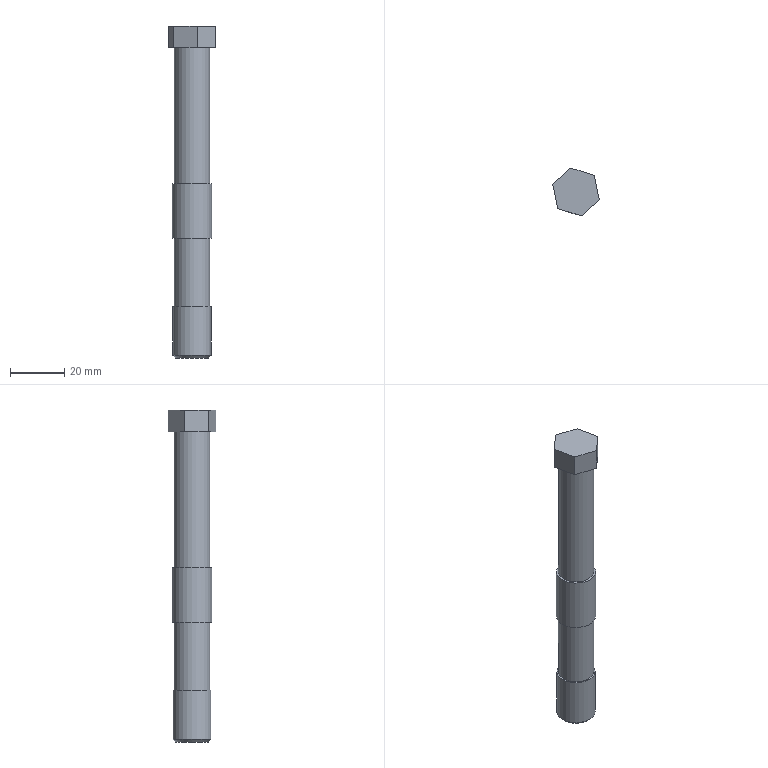Part | NX | features DATUM_CSYS 6, EXTRUDE 4, SKETCH 4, CHAMFER 1, SYMBOLIC_THREAD 1, UNITE 1 | 2 solids | 21 faces | box 17.119 x 17.607 x 122 mm | volume 18493 mm3 | plane 14 | cylinder 6 | cone 1 | commonest cylinder face diameters 13 x3 14.5 x2 14 x1
STEP:
#1=CARTESIAN_POINT('',(6.5,0.,0.));
#2=VERTEX_POINT('',#1);
#3=CARTESIAN_POINT('',(0.,0.,0.));
#4=DIRECTION('',(0.,0.,-1.));
#5=DIRECTION('',(1.,0.,0.));
#6=AXIS2_PLACEMENT_3D('',#3,#4,#5);
#7=CIRCLE('',#6,6.5);
#8=EDGE_CURVE('',#2,#2,#7,.T.);
#9=ORIENTED_EDGE('',*,*,#8,.T.);
#10=EDGE_LOOP('',(#9));
#11=FACE_BOUND('',#10,.T.);
#12=CARTESIAN_POINT('',(-6.5,0.,-50.));
#13=VERTEX_POINT('',#12);
#14=CARTESIAN_POINT('',(0.,0.,-50.));
#15=DIRECTION('',(0.,0.,-1.));
#16=DIRECTION('',(-1.,0.,0.));
#17=AXIS2_PLACEMENT_3D('',#14,#15,#16);
#18=CIRCLE('',#17,6.5);
#19=EDGE_CURVE('',#13,#13,#18,.T.);
#20=ORIENTED_EDGE('',*,*,#19,.F.);
#21=EDGE_LOOP('',(#20));
#22=FACE_BOUND('',#21,.T.);
#23=CARTESIAN_POINT('',(0.,0.,-100.));
#24=DIRECTION('',(0.,0.,1.));
#25=DIRECTION('',(1.,0.,0.));
#26=AXIS2_PLACEMENT_3D('',#23,#24,#25);
#27=CYLINDRICAL_SURFACE('',#26,6.5);
#28=ADVANCED_FACE('',(#11,#22),#27,.T.);
#29=CARTESIAN_POINT('',(1.871,-8.803,0.));
#30=VERTEX_POINT('',#29);
#31=CARTESIAN_POINT('',(8.56,-2.781,0.));
#32=VERTEX_POINT('',#31);
#33=CARTESIAN_POINT('',(1.871,-8.803,0.));
#34=DIRECTION('',(0.7431,0.6691,0.));
#35=VECTOR('',#34,1000.);
#36=LINE('',#33,#35);
#37=EDGE_CURVE('',#30,#32,#36,.T.);
#38=ORIENTED_EDGE('',*,*,#37,.F.);
#39=CARTESIAN_POINT('',(-6.688,-6.022,0.));
#40=VERTEX_POINT('',#39);
#41=CARTESIAN_POINT('',(-6.688,-6.022,0.));
#42=DIRECTION('',(0.9511,-0.309,0.));
#43=VECTOR('',#42,1000.);
#44=LINE('',#41,#43);
#45=EDGE_CURVE('',#40,#30,#44,.T.);
#46=ORIENTED_EDGE('',*,*,#45,.F.);
#47=CARTESIAN_POINT('',(-8.56,2.781,0.));
#48=VERTEX_POINT('',#47);
#49=CARTESIAN_POINT('',(-8.56,2.781,0.));
#50=DIRECTION('',(0.2079,-0.9781,0.));
#51=VECTOR('',#50,1000.);
#52=LINE('',#49,#51);
#53=EDGE_CURVE('',#48,#40,#52,.T.);
#54=ORIENTED_EDGE('',*,*,#53,.F.);
#55=CARTESIAN_POINT('',(-1.871,8.803,0.));
#56=VERTEX_POINT('',#55);
#57=CARTESIAN_POINT('',(-1.871,8.803,0.));
#58=DIRECTION('',(-0.7431,-0.6691,0.));
#59=VECTOR('',#58,1000.);
#60=LINE('',#57,#59);
#61=EDGE_CURVE('',#56,#48,#60,.T.);
#62=ORIENTED_EDGE('',*,*,#61,.F.);
#63=CARTESIAN_POINT('',(6.688,6.022,0.));
#64=VERTEX_POINT('',#63);
#65=CARTESIAN_POINT('',(6.688,6.022,0.));
#66=DIRECTION('',(-0.9511,0.309,0.));
#67=VECTOR('',#66,1000.);
#68=LINE('',#65,#67);
#69=EDGE_CURVE('',#64,#56,#68,.T.);
#70=ORIENTED_EDGE('',*,*,#69,.F.);
#71=CARTESIAN_POINT('',(8.56,-2.781,0.));
#72=DIRECTION('',(-0.2079,0.9781,0.));
#73=VECTOR('',#72,1000.);
#74=LINE('',#71,#73);
#75=EDGE_CURVE('',#32,#64,#74,.T.);
#76=ORIENTED_EDGE('',*,*,#75,.F.);
#77=EDGE_LOOP('',(#38,#46,#54,#62,#70,#76));
#78=FACE_BOUND('',#77,.T.);
#79=ORIENTED_EDGE('',*,*,#8,.F.);
#80=EDGE_LOOP('',(#79));
#81=FACE_BOUND('',#80,.T.);
#82=CARTESIAN_POINT('',(0.,0.,0.));
#83=DIRECTION('',(0.,0.,1.));
#84=DIRECTION('',(1.,0.,0.));
#85=AXIS2_PLACEMENT_3D('',#82,#83,#84);
#86=PLANE('',#85);
#87=ADVANCED_FACE('',(#78,#81),#86,.F.);
#88=ORIENTED_EDGE('',*,*,#37,.T.);
#89=CARTESIAN_POINT('',(8.56,-2.781,8.));
#90=VERTEX_POINT('',#89);
#91=CARTESIAN_POINT('',(8.56,-2.781,8.));
#92=DIRECTION('',(0.,0.,-1.));
#93=VECTOR('',#92,1000.);
#94=LINE('',#91,#93);
#95=EDGE_CURVE('',#90,#32,#94,.T.);
#96=ORIENTED_EDGE('',*,*,#95,.F.);
#97=CARTESIAN_POINT('',(1.871,-8.803,8.));
#98=VERTEX_POINT('',#97);
#99=CARTESIAN_POINT('',(1.871,-8.803,8.));
#100=DIRECTION('',(0.7431,0.6691,0.));
#101=VECTOR('',#100,1000.);
#102=LINE('',#99,#101);
#103=EDGE_CURVE('',#98,#90,#102,.T.);
#104=ORIENTED_EDGE('',*,*,#103,.F.);
#105=CARTESIAN_POINT('',(1.871,-8.803,8.));
#106=DIRECTION('',(0.,0.,-1.));
#107=VECTOR('',#106,1000.);
#108=LINE('',#105,#107);
#109=EDGE_CURVE('',#98,#30,#108,.T.);
#110=ORIENTED_EDGE('',*,*,#109,.T.);
#111=EDGE_LOOP('',(#88,#96,#104,#110));
#112=FACE_BOUND('',#111,.T.);
#113=CARTESIAN_POINT('',(1.871,-8.803,8.));
#114=DIRECTION('',(-0.6691,0.7431,0.));
#115=DIRECTION('',(-0.7431,-0.6691,0.));
#116=AXIS2_PLACEMENT_3D('',#113,#114,#115);
#117=PLANE('',#116);
#118=ADVANCED_FACE('',(#112),#117,.F.);
#119=ORIENTED_EDGE('',*,*,#75,.T.);
#120=CARTESIAN_POINT('',(6.688,6.022,8.));
#121=VERTEX_POINT('',#120);
#122=CARTESIAN_POINT('',(6.688,6.022,8.));
#123=DIRECTION('',(0.,0.,-1.));
#124=VECTOR('',#123,1000.);
#125=LINE('',#122,#124);
#126=EDGE_CURVE('',#121,#64,#125,.T.);
#127=ORIENTED_EDGE('',*,*,#126,.F.);
#128=CARTESIAN_POINT('',(8.56,-2.781,8.));
#129=DIRECTION('',(-0.2079,0.9781,0.));
#130=VECTOR('',#129,1000.);
#131=LINE('',#128,#130);
#132=EDGE_CURVE('',#90,#121,#131,.T.);
#133=ORIENTED_EDGE('',*,*,#132,.F.);
#134=ORIENTED_EDGE('',*,*,#95,.T.);
#135=EDGE_LOOP('',(#119,#127,#133,#134));
#136=FACE_BOUND('',#135,.T.);
#137=CARTESIAN_POINT('',(8.56,-2.781,8.));
#138=DIRECTION('',(-0.9781,-0.2079,0.));
#139=DIRECTION('',(0.2079,-0.9781,0.));
#140=AXIS2_PLACEMENT_3D('',#137,#138,#139);
#141=PLANE('',#140);
#142=ADVANCED_FACE('',(#136),#141,.F.);
#143=ORIENTED_EDGE('',*,*,#69,.T.);
#144=CARTESIAN_POINT('',(-1.871,8.803,8.));
#145=VERTEX_POINT('',#144);
#146=CARTESIAN_POINT('',(-1.871,8.803,8.));
#147=DIRECTION('',(0.,0.,-1.));
#148=VECTOR('',#147,1000.);
#149=LINE('',#146,#148);
#150=EDGE_CURVE('',#145,#56,#149,.T.);
#151=ORIENTED_EDGE('',*,*,#150,.F.);
#152=CARTESIAN_POINT('',(6.688,6.022,8.));
#153=DIRECTION('',(-0.9511,0.309,0.));
#154=VECTOR('',#153,1000.);
#155=LINE('',#152,#154);
#156=EDGE_CURVE('',#121,#145,#155,.T.);
#157=ORIENTED_EDGE('',*,*,#156,.F.);
#158=ORIENTED_EDGE('',*,*,#126,.T.);
#159=EDGE_LOOP('',(#143,#151,#157,#158));
#160=FACE_BOUND('',#159,.T.);
#161=CARTESIAN_POINT('',(6.688,6.022,8.));
#162=DIRECTION('',(-0.309,-0.9511,0.));
#163=DIRECTION('',(0.9511,-0.309,0.));
#164=AXIS2_PLACEMENT_3D('',#161,#162,#163);
#165=PLANE('',#164);
#166=ADVANCED_FACE('',(#160),#165,.F.);
#167=ORIENTED_EDGE('',*,*,#61,.T.);
#168=CARTESIAN_POINT('',(-8.56,2.781,8.));
#169=VERTEX_POINT('',#168);
#170=CARTESIAN_POINT('',(-8.56,2.781,8.));
#171=DIRECTION('',(0.,0.,-1.));
#172=VECTOR('',#171,1000.);
#173=LINE('',#170,#172);
#174=EDGE_CURVE('',#169,#48,#173,.T.);
#175=ORIENTED_EDGE('',*,*,#174,.F.);
#176=CARTESIAN_POINT('',(-1.871,8.803,8.));
#177=DIRECTION('',(-0.7431,-0.6691,0.));
#178=VECTOR('',#177,1000.);
#179=LINE('',#176,#178);
#180=EDGE_CURVE('',#145,#169,#179,.T.);
#181=ORIENTED_EDGE('',*,*,#180,.F.);
#182=ORIENTED_EDGE('',*,*,#150,.T.);
#183=EDGE_LOOP('',(#167,#175,#181,#182));
#184=FACE_BOUND('',#183,.T.);
#185=CARTESIAN_POINT('',(-1.871,8.803,8.));
#186=DIRECTION('',(0.6691,-0.7431,0.));
#187=DIRECTION('',(0.7431,0.6691,0.));
#188=AXIS2_PLACEMENT_3D('',#185,#186,#187);
#189=PLANE('',#188);
#190=ADVANCED_FACE('',(#184),#189,.F.);
#191=ORIENTED_EDGE('',*,*,#53,.T.);
#192=CARTESIAN_POINT('',(-6.688,-6.022,8.));
#193=VERTEX_POINT('',#192);
#194=CARTESIAN_POINT('',(-6.688,-6.022,8.));
#195=DIRECTION('',(0.,0.,-1.));
#196=VECTOR('',#195,1000.);
#197=LINE('',#194,#196);
#198=EDGE_CURVE('',#193,#40,#197,.T.);
#199=ORIENTED_EDGE('',*,*,#198,.F.);
#200=CARTESIAN_POINT('',(-8.56,2.781,8.));
#201=DIRECTION('',(0.2079,-0.9781,0.));
#202=VECTOR('',#201,1000.);
#203=LINE('',#200,#202);
#204=EDGE_CURVE('',#169,#193,#203,.T.);
#205=ORIENTED_EDGE('',*,*,#204,.F.);
#206=ORIENTED_EDGE('',*,*,#174,.T.);
#207=EDGE_LOOP('',(#191,#199,#205,#206));
#208=FACE_BOUND('',#207,.T.);
#209=CARTESIAN_POINT('',(-8.56,2.781,8.));
#210=DIRECTION('',(0.9781,0.2079,0.));
#211=DIRECTION('',(-0.2079,0.9781,0.));
#212=AXIS2_PLACEMENT_3D('',#209,#210,#211);
#213=PLANE('',#212);
#214=ADVANCED_FACE('',(#208),#213,.F.);
#215=ORIENTED_EDGE('',*,*,#45,.T.);
#216=ORIENTED_EDGE('',*,*,#109,.F.);
#217=CARTESIAN_POINT('',(-6.688,-6.022,8.));
#218=DIRECTION('',(0.9511,-0.309,0.));
#219=VECTOR('',#218,1000.);
#220=LINE('',#217,#219);
#221=EDGE_CURVE('',#193,#98,#220,.T.);
#222=ORIENTED_EDGE('',*,*,#221,.F.);
#223=ORIENTED_EDGE('',*,*,#198,.T.);
#224=EDGE_LOOP('',(#215,#216,#222,#223));
#225=FACE_BOUND('',#224,.T.);
#226=CARTESIAN_POINT('',(-6.688,-6.022,8.));
#227=DIRECTION('',(0.309,0.9511,0.));
#228=DIRECTION('',(-0.9511,0.309,0.));
#229=AXIS2_PLACEMENT_3D('',#226,#227,#228);
#230=PLANE('',#229);
#231=ADVANCED_FACE('',(#225),#230,.F.);
#232=ORIENTED_EDGE('',*,*,#103,.T.);
#233=ORIENTED_EDGE('',*,*,#132,.T.);
#234=ORIENTED_EDGE('',*,*,#156,.T.);
#235=ORIENTED_EDGE('',*,*,#180,.T.);
#236=ORIENTED_EDGE('',*,*,#204,.T.);
#237=ORIENTED_EDGE('',*,*,#221,.T.);
#238=EDGE_LOOP('',(#232,#233,#234,#235,#236,#237));
#239=FACE_BOUND('',#238,.T.);
#240=CARTESIAN_POINT('',(0.,0.,8.));
#241=DIRECTION('',(0.,0.,1.));
#242=DIRECTION('',(1.,0.,0.));
#243=AXIS2_PLACEMENT_3D('',#240,#241,#242);
#244=PLANE('',#243);
#245=ADVANCED_FACE('',(#239),#244,.T.);
#246=CARTESIAN_POINT('',(7.25,0.,-50.));
#247=VERTEX_POINT('',#246);
#248=CARTESIAN_POINT('',(0.,0.,-50.));
#249=DIRECTION('',(0.,0.,-1.));
#250=DIRECTION('',(1.,0.,0.));
#251=AXIS2_PLACEMENT_3D('',#248,#249,#250);
#252=CIRCLE('',#251,7.25);
#253=EDGE_CURVE('',#247,#247,#252,.T.);
#254=ORIENTED_EDGE('',*,*,#253,.T.);
#255=EDGE_LOOP('',(#254));
#256=FACE_BOUND('',#255,.T.);
#257=CARTESIAN_POINT('',(7.25,0.,-70.));
#258=VERTEX_POINT('',#257);
#259=CARTESIAN_POINT('',(0.,0.,-70.));
#260=DIRECTION('',(0.,0.,-1.));
#261=DIRECTION('',(1.,0.,0.));
#262=AXIS2_PLACEMENT_3D('',#259,#260,#261);
#263=CIRCLE('',#262,7.25);
#264=EDGE_CURVE('',#258,#258,#263,.T.);
#265=ORIENTED_EDGE('',*,*,#264,.F.);
#266=EDGE_LOOP('',(#265));
#267=FACE_BOUND('',#266,.T.);
#268=CARTESIAN_POINT('',(0.,0.,-50.));
#269=DIRECTION('',(0.,0.,-1.));
#270=DIRECTION('',(-1.,0.,0.));
#271=AXIS2_PLACEMENT_3D('',#268,#269,#270);
#272=CYLINDRICAL_SURFACE('',#271,7.25);
#273=ADVANCED_FACE('',(#256,#267),#272,.T.);
#274=ORIENTED_EDGE('',*,*,#253,.F.);
#275=EDGE_LOOP('',(#274));
#276=FACE_BOUND('',#275,.T.);
#277=ORIENTED_EDGE('',*,*,#19,.T.);
#278=EDGE_LOOP('',(#277));
#279=FACE_BOUND('',#278,.T.);
#280=CARTESIAN_POINT('',(0.,0.,-50.));
#281=DIRECTION('',(0.,0.,-1.));
#282=DIRECTION('',(-1.,0.,0.));
#283=AXIS2_PLACEMENT_3D('',#280,#281,#282);
#284=PLANE('',#283);
#285=ADVANCED_FACE('',(#276,#279),#284,.F.);
#286=ORIENTED_EDGE('',*,*,#264,.T.);
#287=EDGE_LOOP('',(#286));
#288=FACE_BOUND('',#287,.T.);
#289=CARTESIAN_POINT('',(6.5,0.,-70.));
#290=VERTEX_POINT('',#289);
#291=CARTESIAN_POINT('',(0.,0.,-70.));
#292=DIRECTION('',(0.,0.,-1.));
#293=DIRECTION('',(1.,0.,0.));
#294=AXIS2_PLACEMENT_3D('',#291,#292,#293);
#295=CIRCLE('',#294,6.5);
#296=EDGE_CURVE('',#290,#290,#295,.T.);
#297=ORIENTED_EDGE('',*,*,#296,.F.);
#298=EDGE_LOOP('',(#297));
#299=FACE_BOUND('',#298,.T.);
#300=CARTESIAN_POINT('',(0.,0.,-70.));
#301=DIRECTION('',(0.,0.,-1.));
#302=DIRECTION('',(-1.,0.,0.));
#303=AXIS2_PLACEMENT_3D('',#300,#301,#302);
#304=PLANE('',#303);
#305=ADVANCED_FACE('',(#288,#299),#304,.T.);
#306=CARTESIAN_POINT('',(-6.,0.,-114.));
#307=VERTEX_POINT('',#306);
#308=CARTESIAN_POINT('',(0.,0.,-114.));
#309=DIRECTION('',(0.,0.,-1.));
#310=DIRECTION('',(-1.,0.,0.));
#311=AXIS2_PLACEMENT_3D('',#308,#309,#310);
#312=CIRCLE('',#311,6.);
#313=EDGE_CURVE('',#307,#307,#312,.T.);
#314=ORIENTED_EDGE('',*,*,#313,.T.);
#315=EDGE_LOOP('',(#314));
#316=FACE_BOUND('',#315,.T.);
#317=CARTESIAN_POINT('',(0.,0.,-114.));
#318=DIRECTION('',(0.,0.,-1.));
#319=DIRECTION('',(-1.,0.,0.));
#320=AXIS2_PLACEMENT_3D('',#317,#318,#319);
#321=PLANE('',#320);
#322=ADVANCED_FACE('',(#316),#321,.T.);
#323=CARTESIAN_POINT('',(-7.,0.,-113.));
#324=VERTEX_POINT('',#323);
#325=CARTESIAN_POINT('',(0.,0.,-113.));
#326=DIRECTION('',(0.,0.,-1.));
#327=DIRECTION('',(-1.,0.,0.));
#328=AXIS2_PLACEMENT_3D('',#325,#326,#327);
#329=CIRCLE('',#328,7.);
#330=EDGE_CURVE('',#324,#324,#329,.F.);
#331=ORIENTED_EDGE('',*,*,#330,.T.);
#332=EDGE_LOOP('',(#331));
#333=FACE_BOUND('',#332,.T.);
#334=CARTESIAN_POINT('',(7.,0.,-95.));
#335=VERTEX_POINT('',#334);
#336=CARTESIAN_POINT('',(0.,0.,-95.));
#337=DIRECTION('',(0.,0.,-1.));
#338=DIRECTION('',(1.,0.,0.));
#339=AXIS2_PLACEMENT_3D('',#336,#337,#338);
#340=CIRCLE('',#339,7.);
#341=EDGE_CURVE('',#335,#335,#340,.T.);
#342=ORIENTED_EDGE('',*,*,#341,.T.);
#343=EDGE_LOOP('',(#342));
#344=FACE_BOUND('',#343,.T.);
#345=CARTESIAN_POINT('',(0.,0.,-114.));
#346=DIRECTION('',(0.,0.,1.));
#347=DIRECTION('',(1.,0.,0.));
#348=AXIS2_PLACEMENT_3D('',#345,#346,#347);
#349=CYLINDRICAL_SURFACE('',#348,7.);
#350=ADVANCED_FACE('',(#333,#344),#349,.T.);
#351=ORIENTED_EDGE('',*,*,#341,.F.);
#352=EDGE_LOOP('',(#351));
#353=FACE_BOUND('',#352,.T.);
#354=CARTESIAN_POINT('',(-6.5,0.,-95.));
#355=VERTEX_POINT('',#354);
#356=CARTESIAN_POINT('',(0.,0.,-95.));
#357=DIRECTION('',(0.,0.,-1.));
#358=DIRECTION('',(-1.,0.,0.));
#359=AXIS2_PLACEMENT_3D('',#356,#357,#358);
#360=CIRCLE('',#359,6.5);
#361=EDGE_CURVE('',#355,#355,#360,.T.);
#362=ORIENTED_EDGE('',*,*,#361,.T.);
#363=EDGE_LOOP('',(#362));
#364=FACE_BOUND('',#363,.T.);
#365=CARTESIAN_POINT('',(0.,0.,-95.));
#366=DIRECTION('',(0.,0.,-1.));
#367=DIRECTION('',(-1.,0.,0.));
#368=AXIS2_PLACEMENT_3D('',#365,#366,#367);
#369=PLANE('',#368);
#370=ADVANCED_FACE('',(#353,#364),#369,.F.);
#371=ORIENTED_EDGE('',*,*,#296,.T.);
#372=EDGE_LOOP('',(#371));
#373=FACE_BOUND('',#372,.T.);
#374=ORIENTED_EDGE('',*,*,#361,.F.);
#375=EDGE_LOOP('',(#374));
#376=FACE_BOUND('',#375,.T.);
#377=CARTESIAN_POINT('',(0.,0.,-100.));
#378=DIRECTION('',(0.,0.,1.));
#379=DIRECTION('',(1.,0.,0.));
#380=AXIS2_PLACEMENT_3D('',#377,#378,#379);
#381=CYLINDRICAL_SURFACE('',#380,6.5);
#382=ADVANCED_FACE('',(#373,#376),#381,.T.);
#383=ORIENTED_EDGE('',*,*,#330,.F.);
#384=EDGE_LOOP('',(#383));
#385=FACE_BOUND('',#384,.T.);
#386=ORIENTED_EDGE('',*,*,#313,.F.);
#387=EDGE_LOOP('',(#386));
#388=FACE_BOUND('',#387,.T.);
#389=CARTESIAN_POINT('',(0.,0.,-114.));
#390=DIRECTION('',(0.,0.,1.));
#391=DIRECTION('',(1.,0.,0.));
#392=AXIS2_PLACEMENT_3D('',#389,#390,#391);
#393=CONICAL_SURFACE('',#392,6.,0.7854);
#394=ADVANCED_FACE('',(#385,#388),#393,.T.);
#395=CLOSED_SHELL('',(#28,#87,#118,#142,#166,#190,#214,#231,#245,#273,#285,#305,#322,#350,#370,#382,#394));
#396=MANIFOLD_SOLID_BREP('',#395);
#397=CARTESIAN_POINT('',(7.25,0.,-50.));
#398=VERTEX_POINT('',#397);
#399=CARTESIAN_POINT('',(0.,0.,-50.));
#400=DIRECTION('',(0.,0.,-1.));
#401=DIRECTION('',(1.,0.,0.));
#402=AXIS2_PLACEMENT_3D('',#399,#400,#401);
#403=CIRCLE('',#402,7.25);
#404=EDGE_CURVE('',#398,#398,#403,.T.);
#405=ORIENTED_EDGE('',*,*,#404,.T.);
#406=EDGE_LOOP('',(#405));
#407=FACE_BOUND('',#406,.T.);
#408=CARTESIAN_POINT('',(7.25,0.,-70.));
#409=VERTEX_POINT('',#408);
#410=CARTESIAN_POINT('',(0.,0.,-70.));
#411=DIRECTION('',(0.,0.,-1.));
#412=DIRECTION('',(1.,0.,0.));
#413=AXIS2_PLACEMENT_3D('',#410,#411,#412);
#414=CIRCLE('',#413,7.25);
#415=EDGE_CURVE('',#409,#409,#414,.T.);
#416=ORIENTED_EDGE('',*,*,#415,.F.);
#417=EDGE_LOOP('',(#416));
#418=FACE_BOUND('',#417,.T.);
#419=CARTESIAN_POINT('',(0.,0.,-50.));
#420=DIRECTION('',(0.,0.,-1.));
#421=DIRECTION('',(-1.,0.,0.));
#422=AXIS2_PLACEMENT_3D('',#419,#420,#421);
#423=CYLINDRICAL_SURFACE('',#422,7.25);
#424=ADVANCED_FACE('',(#407,#418),#423,.T.);
#425=CARTESIAN_POINT('',(6.5,0.,-50.));
#426=VERTEX_POINT('',#425);
#427=CARTESIAN_POINT('',(0.,0.,-50.));
#428=DIRECTION('',(0.,0.,-1.));
#429=DIRECTION('',(1.,0.,0.));
#430=AXIS2_PLACEMENT_3D('',#427,#428,#429);
#431=CIRCLE('',#430,6.5);
#432=EDGE_CURVE('',#426,#426,#431,.T.);
#433=ORIENTED_EDGE('',*,*,#432,.F.);
#434=EDGE_LOOP('',(#433));
#435=FACE_BOUND('',#434,.T.);
#436=CARTESIAN_POINT('',(6.5,0.,-70.));
#437=VERTEX_POINT('',#436);
#438=CARTESIAN_POINT('',(0.,0.,-70.));
#439=DIRECTION('',(0.,0.,-1.));
#440=DIRECTION('',(1.,0.,0.));
#441=AXIS2_PLACEMENT_3D('',#438,#439,#440);
#442=CIRCLE('',#441,6.5);
#443=EDGE_CURVE('',#437,#437,#442,.T.);
#444=ORIENTED_EDGE('',*,*,#443,.T.);
#445=EDGE_LOOP('',(#444));
#446=FACE_BOUND('',#445,.T.);
#447=CARTESIAN_POINT('',(0.,0.,-50.));
#448=DIRECTION('',(0.,0.,-1.));
#449=DIRECTION('',(-1.,0.,0.));
#450=AXIS2_PLACEMENT_3D('',#447,#448,#449);
#451=CYLINDRICAL_SURFACE('',#450,6.5);
#452=ADVANCED_FACE('',(#435,#446),#451,.F.);
#453=ORIENTED_EDGE('',*,*,#404,.F.);
#454=EDGE_LOOP('',(#453));
#455=FACE_BOUND('',#454,.T.);
#456=ORIENTED_EDGE('',*,*,#432,.T.);
#457=EDGE_LOOP('',(#456));
#458=FACE_BOUND('',#457,.T.);
#459=CARTESIAN_POINT('',(0.,0.,-50.));
#460=DIRECTION('',(0.,0.,-1.));
#461=DIRECTION('',(-1.,0.,0.));
#462=AXIS2_PLACEMENT_3D('',#459,#460,#461);
#463=PLANE('',#462);
#464=ADVANCED_FACE('',(#455,#458),#463,.F.);
#465=ORIENTED_EDGE('',*,*,#415,.T.);
#466=EDGE_LOOP('',(#465));
#467=FACE_BOUND('',#466,.T.);
#468=ORIENTED_EDGE('',*,*,#443,.F.);
#469=EDGE_LOOP('',(#468));
#470=FACE_BOUND('',#469,.T.);
#471=CARTESIAN_POINT('',(0.,0.,-70.));
#472=DIRECTION('',(0.,0.,-1.));
#473=DIRECTION('',(-1.,0.,0.));
#474=AXIS2_PLACEMENT_3D('',#471,#472,#473);
#475=PLANE('',#474);
#476=ADVANCED_FACE('',(#467,#470),#475,.T.);
#477=CLOSED_SHELL('',(#424,#452,#464,#476));
#478=MANIFOLD_SOLID_BREP('',#477);
#479=(LENGTH_UNIT()NAMED_UNIT(*)SI_UNIT(.MILLI.,.METRE.));
#480=UNCERTAINTY_MEASURE_WITH_UNIT(LENGTH_MEASURE(0.00001),#479,'','');
#481=(NAMED_UNIT(*)PLANE_ANGLE_UNIT()SI_UNIT($,.RADIAN.));
#482=(NAMED_UNIT(*)SI_UNIT($,.STERADIAN.)SOLID_ANGLE_UNIT());
#483=(GEOMETRIC_REPRESENTATION_CONTEXT(3)GLOBAL_UNCERTAINTY_ASSIGNED_CONTEXT((#480))GLOBAL_UNIT_ASSIGNED_CONTEXT((#479,#481,#482))REPRESENTATION_CONTEXT('',''));
#484=ADVANCED_BREP_SHAPE_REPRESENTATION('',(#396,#478),#483);